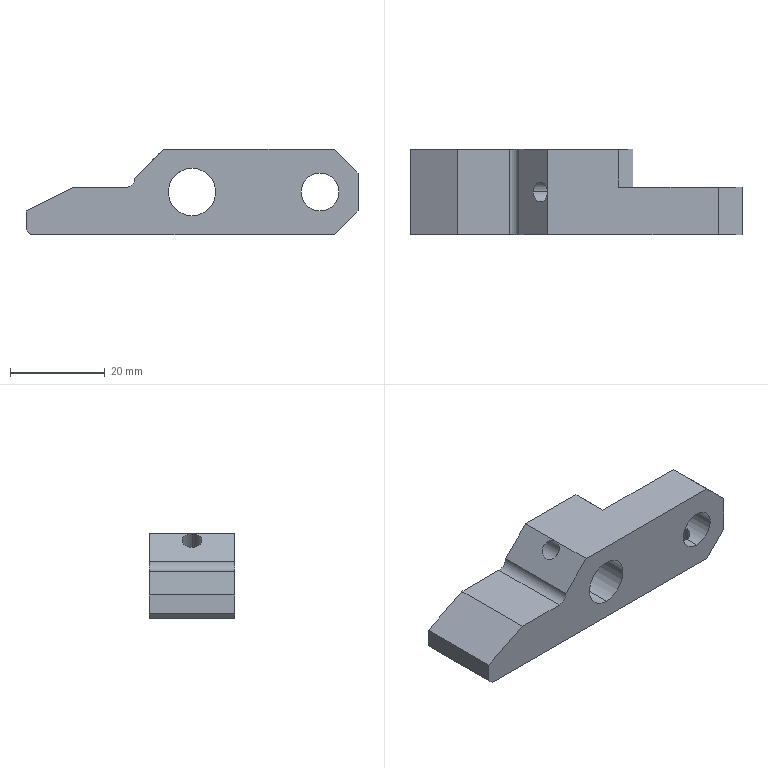Part | SolidWorks | features Chamfer 5, ICE 4, HoleWzd 3, 3DProfileFeature 1, CirPattern 1, Extrusion 1, Fillet 1 | 1 solid | 27 faces | box 70 x 18 x 18 mm | volume 12843 mm3 | plane 16 | cylinder 11 | commonest cylinder face diameters 4.2 x6 8 x2 10 x2 4 x1
STEP:
#1=CARTESIAN_POINT('',(-12.194,9.,1.724));
#2=VERTEX_POINT('',#1);
#3=CARTESIAN_POINT('',(-9.224,9.,4.694));
#4=VERTEX_POINT('',#3);
#5=CARTESIAN_POINT('',(-12.194,9.,1.724));
#6=CARTESIAN_POINT('',(-12.194,8.862,1.724));
#7=CARTESIAN_POINT('',(-12.188,8.721,1.738));
#8=CARTESIAN_POINT('',(-12.167,8.449,1.794));
#9=CARTESIAN_POINT('',(-12.151,8.318,1.836));
#10=CARTESIAN_POINT('',(-12.086,7.937,1.995));
#11=CARTESIAN_POINT('',(-12.02,7.708,2.147));
#12=CARTESIAN_POINT('',(-11.879,7.418,2.416));
#13=CARTESIAN_POINT('',(-11.826,7.332,2.511));
#14=CARTESIAN_POINT('',(-11.705,7.181,2.708));
#15=CARTESIAN_POINT('',(-11.636,7.115,2.813));
#16=CARTESIAN_POINT('',(-11.486,7.009,3.021));
#17=CARTESIAN_POINT('',(-11.405,6.969,3.126));
#18=CARTESIAN_POINT('',(-11.229,6.914,3.334));
#19=CARTESIAN_POINT('',(-11.134,6.9,3.437));
#20=CARTESIAN_POINT('',(-10.84,6.9,3.731));
#21=CARTESIAN_POINT('',(-10.625,6.956,3.911));
#22=CARTESIAN_POINT('',(-10.313,7.115,4.136));
#23=CARTESIAN_POINT('',(-10.208,7.181,4.205));
#24=CARTESIAN_POINT('',(-10.01,7.333,4.326));
#25=CARTESIAN_POINT('',(-9.915,7.419,4.379));
#26=CARTESIAN_POINT('',(-9.736,7.612,4.473));
#27=CARTESIAN_POINT('',(-9.653,7.718,4.513));
#28=CARTESIAN_POINT('',(-9.507,7.943,4.58));
#29=CARTESIAN_POINT('',(-9.443,8.063,4.608));
#30=CARTESIAN_POINT('',(-9.335,8.319,4.651));
#31=CARTESIAN_POINT('',(-9.294,8.45,4.667));
#32=CARTESIAN_POINT('',(-9.238,8.72,4.688));
#33=CARTESIAN_POINT('',(-9.224,8.86,4.694));
#34=CARTESIAN_POINT('',(-9.224,9.,4.694));
#35=B_SPLINE_CURVE_WITH_KNOTS('',3,(#5,#6,#7,#8,#9,#10,#11,#12,#13,#14,#15,#16,#17,#18,#19,#20,#21,#22,#23,#24,#25,#26,#27,#28,#29,#30,#31,#32,#33,#34),.UNSPECIFIED.,.F.,.F.,(4,2,2,2,2,2,2,2,2,2,2,2,2,2,4),(0.006643,0.007058,0.007473,0.008303,0.008717,0.009132,0.009547,0.009962,0.01079,0.01121,0.01162,0.01204,0.01245,0.01287,0.01328),.UNSPECIFIED.);
#36=EDGE_CURVE('',#2,#4,#35,.T.);
#37=ORIENTED_EDGE('',*,*,#36,.F.);
#38=CARTESIAN_POINT('',(-16.485,9.,6.015));
#39=VERTEX_POINT('',#38);
#40=CARTESIAN_POINT('',(-15.349,9.,4.879));
#41=DIRECTION('',(-0.7071,0.,0.7071));
#42=VECTOR('',#41,1000.);
#43=LINE('',#40,#42);
#44=EDGE_CURVE('',#2,#39,#43,.T.);
#45=ORIENTED_EDGE('',*,*,#44,.T.);
#46=CARTESIAN_POINT('',(-13.515,9.,8.985));
#47=VERTEX_POINT('',#46);
#48=CARTESIAN_POINT('',(-15.,9.,7.5));
#49=DIRECTION('',(-0.7071,0.,0.7071));
#50=DIRECTION('',(0.7071,0.,0.7071));
#51=AXIS2_PLACEMENT_3D('',#48,#49,#50);
#52=CIRCLE('',#51,2.1);
#53=EDGE_CURVE('',#39,#47,#52,.T.);
#54=ORIENTED_EDGE('',*,*,#53,.T.);
#55=CARTESIAN_POINT('',(-12.379,9.,7.849));
#56=DIRECTION('',(-0.7071,0.,0.7071));
#57=VECTOR('',#56,1000.);
#58=LINE('',#55,#57);
#59=EDGE_CURVE('',#4,#47,#58,.T.);
#60=ORIENTED_EDGE('',*,*,#59,.F.);
#61=EDGE_LOOP('',(#37,#45,#54,#60));
#62=FACE_OUTER_BOUND('',#61,.T.);
#63=CARTESIAN_POINT('',(-13.864,9.,6.364));
#64=DIRECTION('',(-0.7071,0.,0.7071));
#65=DIRECTION('',(0.7071,0.,0.7071));
#66=AXIS2_PLACEMENT_3D('',#63,#64,#65);
#67=CYLINDRICAL_SURFACE('',#66,2.1);
#68=ADVANCED_FACE('',(#62),#67,.F.);
#69=CARTESIAN_POINT('',(-5.4,9.,-4.538));
#70=VERTEX_POINT('',#69);
#71=CARTESIAN_POINT('',(-7.5,6.9,-5.));
#72=VERTEX_POINT('',#71);
#73=CARTESIAN_POINT('',(-5.4,9.,-4.538));
#74=CARTESIAN_POINT('',(-5.4,8.862,-4.538));
#75=CARTESIAN_POINT('',(-5.414,8.721,-4.544));
#76=CARTESIAN_POINT('',(-5.469,8.449,-4.569));
#77=CARTESIAN_POINT('',(-5.509,8.318,-4.587));
#78=CARTESIAN_POINT('',(-5.668,7.937,-4.654));
#79=CARTESIAN_POINT('',(-5.822,7.708,-4.715));
#80=CARTESIAN_POINT('',(-6.112,7.418,-4.805));
#81=CARTESIAN_POINT('',(-6.217,7.332,-4.834));
#82=CARTESIAN_POINT('',(-6.442,7.181,-4.888));
#83=CARTESIAN_POINT('',(-6.565,7.115,-4.913));
#84=CARTESIAN_POINT('',(-6.818,7.009,-4.955));
#85=CARTESIAN_POINT('',(-6.949,6.969,-4.971));
#86=CARTESIAN_POINT('',(-7.221,6.914,-4.994));
#87=CARTESIAN_POINT('',(-7.362,6.9,-5.));
#88=CARTESIAN_POINT('',(-7.5,6.9,-5.));
#89=B_SPLINE_CURVE_WITH_KNOTS('',3,(#73,#74,#75,#76,#77,#78,#79,#80,#81,#82,#83,#84,#85,#86,#87,#88),.UNSPECIFIED.,.F.,.F.,(4,2,2,2,2,2,2,4),(0.006643,0.007058,0.007473,0.008303,0.008718,0.009133,0.009547,0.009962),.UNSPECIFIED.);
#90=EDGE_CURVE('',#70,#72,#89,.T.);
#91=ORIENTED_EDGE('',*,*,#90,.F.);
#92=CARTESIAN_POINT('',(-5.4,9.,-9.));
#93=VERTEX_POINT('',#92);
#94=CARTESIAN_POINT('',(-5.4,9.,-9.));
#95=DIRECTION('',(0.,0.,-1.));
#96=VECTOR('',#95,1000.);
#97=LINE('',#94,#96);
#98=EDGE_CURVE('',#70,#93,#97,.T.);
#99=ORIENTED_EDGE('',*,*,#98,.T.);
#100=CARTESIAN_POINT('',(-9.6,9.,-9.));
#101=VERTEX_POINT('',#100);
#102=CARTESIAN_POINT('',(-7.5,9.,-9.));
#103=DIRECTION('',(0.,0.,-1.));
#104=DIRECTION('',(-1.,0.,0.));
#105=AXIS2_PLACEMENT_3D('',#102,#103,#104);
#106=CIRCLE('',#105,2.1);
#107=EDGE_CURVE('',#93,#101,#106,.T.);
#108=ORIENTED_EDGE('',*,*,#107,.T.);
#109=CARTESIAN_POINT('',(-9.6,9.,-4.538));
#110=VERTEX_POINT('',#109);
#111=CARTESIAN_POINT('',(-9.6,9.,-9.));
#112=DIRECTION('',(0.,0.,-1.));
#113=VECTOR('',#112,1000.);
#114=LINE('',#111,#113);
#115=EDGE_CURVE('',#110,#101,#114,.T.);
#116=ORIENTED_EDGE('',*,*,#115,.F.);
#117=CARTESIAN_POINT('',(-7.5,6.9,-5.));
#118=CARTESIAN_POINT('',(-7.777,6.9,-5.));
#119=CARTESIAN_POINT('',(-8.056,6.956,-4.976));
#120=CARTESIAN_POINT('',(-8.436,7.115,-4.913));
#121=CARTESIAN_POINT('',(-8.558,7.181,-4.888));
#122=CARTESIAN_POINT('',(-8.784,7.333,-4.834));
#123=CARTESIAN_POINT('',(-8.889,7.419,-4.804));
#124=CARTESIAN_POINT('',(-9.082,7.612,-4.744));
#125=CARTESIAN_POINT('',(-9.169,7.718,-4.714));
#126=CARTESIAN_POINT('',(-9.32,7.943,-4.658));
#127=CARTESIAN_POINT('',(-9.385,8.063,-4.632));
#128=CARTESIAN_POINT('',(-9.491,8.319,-4.587));
#129=CARTESIAN_POINT('',(-9.531,8.45,-4.569));
#130=CARTESIAN_POINT('',(-9.586,8.72,-4.544));
#131=CARTESIAN_POINT('',(-9.6,8.86,-4.538));
#132=CARTESIAN_POINT('',(-9.6,9.,-4.538));
#133=B_SPLINE_CURVE_WITH_KNOTS('',3,(#117,#118,#119,#120,#121,#122,#123,#124,#125,#126,#127,#128,#129,#130,#131,#132),.UNSPECIFIED.,.F.,.F.,(4,2,2,2,2,2,2,4),(0.009962,0.01079,0.01121,0.01162,0.01204,0.01245,0.01287,0.01328),.UNSPECIFIED.);
#134=EDGE_CURVE('',#72,#110,#133,.T.);
#135=ORIENTED_EDGE('',*,*,#134,.F.);
#136=EDGE_LOOP('',(#91,#99,#108,#116,#135));
#137=FACE_OUTER_BOUND('',#136,.T.);
#138=CARTESIAN_POINT('',(-7.5,9.,-9.));
#139=DIRECTION('',(0.,0.,-1.));
#140=DIRECTION('',(-1.,0.,0.));
#141=AXIS2_PLACEMENT_3D('',#138,#139,#140);
#142=CYLINDRICAL_SURFACE('',#141,2.1);
#143=ADVANCED_FACE('',(#137),#142,.F.);
#144=CARTESIAN_POINT('',(19.5,2.9,-4.));
#145=VERTEX_POINT('',#144);
#146=CARTESIAN_POINT('',(21.6,5.,-3.404));
#147=VERTEX_POINT('',#146);
#148=CARTESIAN_POINT('',(19.5,2.9,-4.));
#149=CARTESIAN_POINT('',(19.64,2.9,-4.));
#150=CARTESIAN_POINT('',(19.782,2.914,-3.992));
#151=CARTESIAN_POINT('',(20.054,2.97,-3.964));
#152=CARTESIAN_POINT('',(20.187,3.011,-3.943));
#153=CARTESIAN_POINT('',(20.443,3.118,-3.89));
#154=CARTESIAN_POINT('',(20.563,3.184,-3.858));
#155=CARTESIAN_POINT('',(20.788,3.335,-3.789));
#156=CARTESIAN_POINT('',(20.893,3.423,-3.751));
#157=CARTESIAN_POINT('',(21.083,3.614,-3.675));
#158=CARTESIAN_POINT('',(21.168,3.718,-3.636));
#159=CARTESIAN_POINT('',(21.32,3.943,-3.563));
#160=CARTESIAN_POINT('',(21.385,4.064,-3.529));
#161=CARTESIAN_POINT('',(21.542,4.44,-3.441));
#162=CARTESIAN_POINT('',(21.6,4.721,-3.404));
#163=CARTESIAN_POINT('',(21.6,5.,-3.404));
#164=B_SPLINE_CURVE_WITH_KNOTS('',3,(#148,#149,#150,#151,#152,#153,#154,#155,#156,#157,#158,#159,#160,#161,#162,#163),.UNSPECIFIED.,.F.,.F.,(4,2,2,2,2,2,2,4),(0.006693,0.007111,0.007529,0.007947,0.008365,0.008783,0.0092,0.01004),.UNSPECIFIED.);
#165=EDGE_CURVE('',#145,#147,#164,.T.);
#166=ORIENTED_EDGE('',*,*,#165,.T.);
#167=CARTESIAN_POINT('',(21.6,5.,-9.));
#168=VERTEX_POINT('',#167);
#169=CARTESIAN_POINT('',(21.6,5.,-9.));
#170=DIRECTION('',(0.,0.,-1.));
#171=VECTOR('',#170,1000.);
#172=LINE('',#169,#171);
#173=EDGE_CURVE('',#147,#168,#172,.T.);
#174=ORIENTED_EDGE('',*,*,#173,.T.);
#175=CARTESIAN_POINT('',(17.4,5.,-9.));
#176=VERTEX_POINT('',#175);
#177=CARTESIAN_POINT('',(19.5,5.,-9.));
#178=DIRECTION('',(0.,0.,-1.));
#179=DIRECTION('',(-1.,0.,0.));
#180=AXIS2_PLACEMENT_3D('',#177,#178,#179);
#181=CIRCLE('',#180,2.1);
#182=EDGE_CURVE('',#168,#176,#181,.T.);
#183=ORIENTED_EDGE('',*,*,#182,.T.);
#184=CARTESIAN_POINT('',(17.4,5.,-3.404));
#185=VERTEX_POINT('',#184);
#186=CARTESIAN_POINT('',(17.4,5.,-9.));
#187=DIRECTION('',(0.,0.,-1.));
#188=VECTOR('',#187,1000.);
#189=LINE('',#186,#188);
#190=EDGE_CURVE('',#185,#176,#189,.T.);
#191=ORIENTED_EDGE('',*,*,#190,.F.);
#192=CARTESIAN_POINT('',(17.4,5.,-3.404));
#193=CARTESIAN_POINT('',(17.4,4.86,-3.404));
#194=CARTESIAN_POINT('',(17.414,4.718,-3.413));
#195=CARTESIAN_POINT('',(17.47,4.446,-3.446));
#196=CARTESIAN_POINT('',(17.511,4.313,-3.471));
#197=CARTESIAN_POINT('',(17.617,4.059,-3.53));
#198=CARTESIAN_POINT('',(17.682,3.94,-3.564));
#199=CARTESIAN_POINT('',(17.834,3.715,-3.637));
#200=CARTESIAN_POINT('',(17.92,3.61,-3.676));
#201=CARTESIAN_POINT('',(18.205,3.325,-3.79));
#202=CARTESIAN_POINT('',(18.436,3.169,-3.864));
#203=CARTESIAN_POINT('',(18.814,3.011,-3.943));
#204=CARTESIAN_POINT('',(18.948,2.969,-3.964));
#205=CARTESIAN_POINT('',(19.222,2.914,-3.993));
#206=CARTESIAN_POINT('',(19.36,2.9,-4.));
#207=CARTESIAN_POINT('',(19.5,2.9,-4.));
#208=B_SPLINE_CURVE_WITH_KNOTS('',3,(#192,#193,#194,#195,#196,#197,#198,#199,#200,#201,#202,#203,#204,#205,#206,#207),.UNSPECIFIED.,.F.,.F.,(4,2,2,2,2,2,2,4),(0.003349,0.003767,0.004185,0.004603,0.005021,0.005857,0.006275,0.006693),.UNSPECIFIED.);
#209=EDGE_CURVE('',#185,#145,#208,.T.);
#210=ORIENTED_EDGE('',*,*,#209,.T.);
#211=EDGE_LOOP('',(#166,#174,#183,#191,#210));
#212=FACE_OUTER_BOUND('',#211,.T.);
#213=CARTESIAN_POINT('',(19.5,5.,-9.));
#214=DIRECTION('',(0.,0.,-1.));
#215=DIRECTION('',(-1.,0.,0.));
#216=AXIS2_PLACEMENT_3D('',#213,#214,#215);
#217=CYLINDRICAL_SURFACE('',#216,2.1);
#218=ADVANCED_FACE('',(#212),#217,.F.);
#219=CARTESIAN_POINT('',(-9.224,9.,4.694));
#220=CARTESIAN_POINT('',(-9.224,9.141,4.694));
#221=CARTESIAN_POINT('',(-9.238,9.278,4.688));
#222=CARTESIAN_POINT('',(-9.294,9.549,4.667));
#223=CARTESIAN_POINT('',(-9.336,9.683,4.651));
#224=CARTESIAN_POINT('',(-9.442,9.936,4.608));
#225=CARTESIAN_POINT('',(-9.506,10.056,4.58));
#226=CARTESIAN_POINT('',(-9.654,10.283,4.513));
#227=CARTESIAN_POINT('',(-9.737,10.389,4.473));
#228=CARTESIAN_POINT('',(-10.003,10.676,4.333));
#229=CARTESIAN_POINT('',(-10.209,10.832,4.211));
#230=CARTESIAN_POINT('',(-10.52,10.99,3.987));
#231=CARTESIAN_POINT('',(-10.627,11.032,3.904));
#232=CARTESIAN_POINT('',(-10.835,11.086,3.728));
#233=CARTESIAN_POINT('',(-10.936,11.1,3.635));
#234=CARTESIAN_POINT('',(-11.133,11.1,3.438));
#235=CARTESIAN_POINT('',(-11.228,11.086,3.334));
#236=CARTESIAN_POINT('',(-11.404,11.032,3.127));
#237=CARTESIAN_POINT('',(-11.486,10.991,3.022));
#238=CARTESIAN_POINT('',(-11.637,10.884,2.811));
#239=CARTESIAN_POINT('',(-11.705,10.819,2.708));
#240=CARTESIAN_POINT('',(-11.826,10.667,2.51));
#241=CARTESIAN_POINT('',(-11.88,10.579,2.413));
#242=CARTESIAN_POINT('',(-11.973,10.387,2.236));
#243=CARTESIAN_POINT('',(-12.013,10.283,2.154));
#244=CARTESIAN_POINT('',(-12.081,10.056,2.006));
#245=CARTESIAN_POINT('',(-12.108,9.934,1.941));
#246=CARTESIAN_POINT('',(-12.173,9.556,1.783));
#247=CARTESIAN_POINT('',(-12.194,9.277,1.724));
#248=CARTESIAN_POINT('',(-12.194,9.,1.724));
#249=B_SPLINE_CURVE_WITH_KNOTS('',3,(#219,#220,#221,#222,#223,#224,#225,#226,#227,#228,#229,#230,#231,#232,#233,#234,#235,#236,#237,#238,#239,#240,#241,#242,#243,#244,#245,#246,#247,#248),.UNSPECIFIED.,.F.,.F.,(4,2,2,2,2,2,2,2,2,2,2,2,2,2,4),(0.,0.0004152,0.0008304,0.001246,0.001661,0.002491,0.002906,0.003322,0.003737,0.004152,0.004567,0.004982,0.005398,0.005813,0.006643),.UNSPECIFIED.);
#250=EDGE_CURVE('',#4,#2,#249,.T.);
#251=ORIENTED_EDGE('',*,*,#250,.T.);
#252=ORIENTED_EDGE('',*,*,#36,.T.);
#253=EDGE_LOOP('',(#251,#252));
#254=FACE_BOUND('',#253,.T.);
#255=CARTESIAN_POINT('',(-7.5,0.,5.));
#256=VERTEX_POINT('',#255);
#257=CARTESIAN_POINT('',(-7.5,0.,-5.));
#258=VERTEX_POINT('',#257);
#259=CARTESIAN_POINT('',(-7.5,0.,0.));
#260=DIRECTION('',(0.,-1.,0.));
#261=DIRECTION('',(0.,0.,-1.));
#262=AXIS2_PLACEMENT_3D('',#259,#260,#261);
#263=CIRCLE('',#262,5.);
#264=EDGE_CURVE('',#256,#258,#263,.T.);
#265=ORIENTED_EDGE('',*,*,#264,.T.);
#266=CARTESIAN_POINT('',(-7.5,-9.,-5.));
#267=DIRECTION('',(0.,1.,0.));
#268=VECTOR('',#267,1000.);
#269=LINE('',#266,#268);
#270=EDGE_CURVE('',#258,#72,#269,.T.);
#271=ORIENTED_EDGE('',*,*,#270,.T.);
#272=ORIENTED_EDGE('',*,*,#134,.T.);
#273=CARTESIAN_POINT('',(-7.5,11.1,-5.));
#274=VERTEX_POINT('',#273);
#275=CARTESIAN_POINT('',(-9.6,9.,-4.538));
#276=CARTESIAN_POINT('',(-9.6,9.141,-4.538));
#277=CARTESIAN_POINT('',(-9.586,9.278,-4.544));
#278=CARTESIAN_POINT('',(-9.532,9.549,-4.569));
#279=CARTESIAN_POINT('',(-9.49,9.683,-4.587));
#280=CARTESIAN_POINT('',(-9.385,9.937,-4.632));
#281=CARTESIAN_POINT('',(-9.32,10.057,-4.658));
#282=CARTESIAN_POINT('',(-9.168,10.284,-4.714));
#283=CARTESIAN_POINT('',(-9.08,10.39,-4.745));
#284=CARTESIAN_POINT('',(-8.793,10.677,-4.834));
#285=CARTESIAN_POINT('',(-8.561,10.833,-4.893));
#286=CARTESIAN_POINT('',(-8.183,10.991,-4.955));
#287=CARTESIAN_POINT('',(-8.049,11.032,-4.972));
#288=CARTESIAN_POINT('',(-7.776,11.086,-4.994));
#289=CARTESIAN_POINT('',(-7.639,11.1,-5.));
#290=CARTESIAN_POINT('',(-7.5,11.1,-5.));
#291=B_SPLINE_CURVE_WITH_KNOTS('',3,(#275,#276,#277,#278,#279,#280,#281,#282,#283,#284,#285,#286,#287,#288,#289,#290),.UNSPECIFIED.,.F.,.F.,(4,2,2,2,2,2,2,4),(0.,0.0004153,0.0008307,0.001246,0.001661,0.002492,0.002907,0.003323),.UNSPECIFIED.);
#292=EDGE_CURVE('',#110,#274,#291,.T.);
#293=ORIENTED_EDGE('',*,*,#292,.T.);
#294=CARTESIAN_POINT('',(-7.5,18.,-5.));
#295=VERTEX_POINT('',#294);
#296=CARTESIAN_POINT('',(-7.5,-9.,-5.));
#297=DIRECTION('',(0.,1.,0.));
#298=VECTOR('',#297,1000.);
#299=LINE('',#296,#298);
#300=EDGE_CURVE('',#274,#295,#299,.T.);
#301=ORIENTED_EDGE('',*,*,#300,.T.);
#302=CARTESIAN_POINT('',(-7.5,18.,5.));
#303=VERTEX_POINT('',#302);
#304=CARTESIAN_POINT('',(-7.5,18.,0.));
#305=DIRECTION('',(0.,1.,0.));
#306=DIRECTION('',(0.,0.,1.));
#307=AXIS2_PLACEMENT_3D('',#304,#305,#306);
#308=CIRCLE('',#307,5.);
#309=EDGE_CURVE('',#295,#303,#308,.T.);
#310=ORIENTED_EDGE('',*,*,#309,.T.);
#311=CARTESIAN_POINT('',(-7.5,-9.,5.));
#312=DIRECTION('',(0.,1.,0.));
#313=VECTOR('',#312,1000.);
#314=LINE('',#311,#313);
#315=EDGE_CURVE('',#256,#303,#314,.T.);
#316=ORIENTED_EDGE('',*,*,#315,.F.);
#317=EDGE_LOOP('',(#265,#271,#272,#293,#301,#310,#316));
#318=FACE_OUTER_BOUND('',#317,.T.);
#319=CARTESIAN_POINT('',(-7.5,-9.,0.));
#320=DIRECTION('',(0.,1.,0.));
#321=DIRECTION('',(0.,0.,1.));
#322=AXIS2_PLACEMENT_3D('',#319,#320,#321);
#323=CYLINDRICAL_SURFACE('',#322,5.);
#324=ADVANCED_FACE('',(#254,#318),#323,.F.);
#325=CARTESIAN_POINT('',(19.5,10.,-4.));
#326=VERTEX_POINT('',#325);
#327=CARTESIAN_POINT('',(19.5,10.,4.));
#328=VERTEX_POINT('',#327);
#329=CARTESIAN_POINT('',(19.5,10.,0.));
#330=DIRECTION('',(0.,1.,0.));
#331=DIRECTION('',(0.,0.,1.));
#332=AXIS2_PLACEMENT_3D('',#329,#330,#331);
#333=CIRCLE('',#332,4.);
#334=EDGE_CURVE('',#326,#328,#333,.T.);
#335=ORIENTED_EDGE('',*,*,#334,.T.);
#336=CARTESIAN_POINT('',(19.5,0.,4.));
#337=VERTEX_POINT('',#336);
#338=CARTESIAN_POINT('',(19.5,10.,4.));
#339=DIRECTION('',(0.,-1.,0.));
#340=VECTOR('',#339,1000.);
#341=LINE('',#338,#340);
#342=EDGE_CURVE('',#328,#337,#341,.T.);
#343=ORIENTED_EDGE('',*,*,#342,.T.);
#344=CARTESIAN_POINT('',(19.5,0.,-4.));
#345=VERTEX_POINT('',#344);
#346=CARTESIAN_POINT('',(19.5,0.,0.));
#347=DIRECTION('',(0.,1.,0.));
#348=DIRECTION('',(0.,0.,1.));
#349=AXIS2_PLACEMENT_3D('',#346,#347,#348);
#350=CIRCLE('',#349,4.);
#351=EDGE_CURVE('',#345,#337,#350,.T.);
#352=ORIENTED_EDGE('',*,*,#351,.F.);
#353=CARTESIAN_POINT('',(19.5,10.,-4.));
#354=DIRECTION('',(0.,-1.,0.));
#355=VECTOR('',#354,1000.);
#356=LINE('',#353,#355);
#357=EDGE_CURVE('',#145,#345,#356,.T.);
#358=ORIENTED_EDGE('',*,*,#357,.F.);
#359=ORIENTED_EDGE('',*,*,#209,.F.);
#360=CARTESIAN_POINT('',(19.5,7.1,-4.));
#361=VERTEX_POINT('',#360);
#362=CARTESIAN_POINT('',(19.5,7.1,-4.));
#363=CARTESIAN_POINT('',(19.358,7.1,-4.));
#364=CARTESIAN_POINT('',(19.219,7.086,-3.992));
#365=CARTESIAN_POINT('',(18.947,7.031,-3.964));
#366=CARTESIAN_POINT('',(18.812,6.989,-3.943));
#367=CARTESIAN_POINT('',(18.432,6.829,-3.863));
#368=CARTESIAN_POINT('',(18.202,6.673,-3.789));
#369=CARTESIAN_POINT('',(17.917,6.387,-3.675));
#370=CARTESIAN_POINT('',(17.831,6.282,-3.636));
#371=CARTESIAN_POINT('',(17.68,6.056,-3.563));
#372=CARTESIAN_POINT('',(17.616,5.937,-3.529));
#373=CARTESIAN_POINT('',(17.51,5.685,-3.471));
#374=CARTESIAN_POINT('',(17.469,5.551,-3.446));
#375=CARTESIAN_POINT('',(17.414,5.278,-3.413));
#376=CARTESIAN_POINT('',(17.4,5.14,-3.404));
#377=CARTESIAN_POINT('',(17.4,5.,-3.404));
#378=B_SPLINE_CURVE_WITH_KNOTS('',3,(#362,#363,#364,#365,#366,#367,#368,#369,#370,#371,#372,#373,#374,#375,#376,#377),.UNSPECIFIED.,.F.,.F.,(4,2,2,2,2,2,2,4),(0.,0.0004186,0.0008373,0.001675,0.002093,0.002512,0.00293,0.003349),.UNSPECIFIED.);
#379=EDGE_CURVE('',#361,#185,#378,.T.);
#380=ORIENTED_EDGE('',*,*,#379,.F.);
#381=CARTESIAN_POINT('',(19.5,10.,-4.));
#382=DIRECTION('',(0.,-1.,0.));
#383=VECTOR('',#382,1000.);
#384=LINE('',#381,#383);
#385=EDGE_CURVE('',#326,#361,#384,.T.);
#386=ORIENTED_EDGE('',*,*,#385,.F.);
#387=EDGE_LOOP('',(#335,#343,#352,#358,#359,#380,#386));
#388=FACE_OUTER_BOUND('',#387,.T.);
#389=CARTESIAN_POINT('',(19.5,10.,0.));
#390=DIRECTION('',(0.,-1.,0.));
#391=DIRECTION('',(0.,0.,-1.));
#392=AXIS2_PLACEMENT_3D('',#389,#390,#391);
#393=CYLINDRICAL_SURFACE('',#392,4.);
#394=ADVANCED_FACE('',(#388),#393,.F.);
#395=ORIENTED_EDGE('',*,*,#334,.F.);
#396=CARTESIAN_POINT('',(19.5,10.,0.));
#397=DIRECTION('',(0.,1.,0.));
#398=DIRECTION('',(0.,0.,1.));
#399=AXIS2_PLACEMENT_3D('',#396,#397,#398);
#400=CIRCLE('',#399,4.);
#401=EDGE_CURVE('',#328,#326,#400,.T.);
#402=ORIENTED_EDGE('',*,*,#401,.F.);
#403=EDGE_LOOP('',(#395,#402));
#404=FACE_BOUND('',#403,.T.);
#405=CARTESIAN_POINT('',(27.5,10.,4.));
#406=VERTEX_POINT('',#405);
#407=CARTESIAN_POINT('',(27.5,10.,-4.));
#408=VERTEX_POINT('',#407);
#409=CARTESIAN_POINT('',(27.5,10.,-9.));
#410=DIRECTION('',(0.,0.,-1.));
#411=VECTOR('',#410,1000.);
#412=LINE('',#409,#411);
#413=EDGE_CURVE('',#406,#408,#412,.T.);
#414=ORIENTED_EDGE('',*,*,#413,.T.);
#415=CARTESIAN_POINT('',(22.5,10.,-9.));
#416=VERTEX_POINT('',#415);
#417=CARTESIAN_POINT('',(22.5,10.,-9.));
#418=DIRECTION('',(-0.7071,0.,-0.7071));
#419=VECTOR('',#418,1000.);
#420=LINE('',#417,#419);
#421=EDGE_CURVE('',#408,#416,#420,.T.);
#422=ORIENTED_EDGE('',*,*,#421,.T.);
#423=CARTESIAN_POINT('',(1.5,10.,-9.));
#424=VERTEX_POINT('',#423);
#425=CARTESIAN_POINT('',(27.5,10.,-9.));
#426=DIRECTION('',(-1.,0.,0.));
#427=VECTOR('',#426,1000.);
#428=LINE('',#425,#427);
#429=EDGE_CURVE('',#416,#424,#428,.T.);
#430=ORIENTED_EDGE('',*,*,#429,.T.);
#431=CARTESIAN_POINT('',(4.5,10.,-6.));
#432=VERTEX_POINT('',#431);
#433=CARTESIAN_POINT('',(5.25,10.,-5.25));
#434=DIRECTION('',(0.7071,0.,0.7071));
#435=VECTOR('',#434,1000.);
#436=LINE('',#433,#435);
#437=EDGE_CURVE('',#424,#432,#436,.T.);
#438=ORIENTED_EDGE('',*,*,#437,.T.);
#439=CARTESIAN_POINT('',(4.5,10.,6.));
#440=VERTEX_POINT('',#439);
#441=CARTESIAN_POINT('',(4.5,10.,41.985));
#442=DIRECTION('',(0.,0.,-1.));
#443=VECTOR('',#442,1000.);
#444=LINE('',#441,#443);
#445=EDGE_CURVE('',#440,#432,#444,.T.);
#446=ORIENTED_EDGE('',*,*,#445,.F.);
#447=CARTESIAN_POINT('',(1.5,10.,9.));
#448=VERTEX_POINT('',#447);
#449=CARTESIAN_POINT('',(5.25,10.,5.25));
#450=DIRECTION('',(-0.7071,0.,0.7071));
#451=VECTOR('',#450,1000.);
#452=LINE('',#449,#451);
#453=EDGE_CURVE('',#440,#448,#452,.T.);
#454=ORIENTED_EDGE('',*,*,#453,.T.);
#455=CARTESIAN_POINT('',(22.5,10.,9.));
#456=VERTEX_POINT('',#455);
#457=CARTESIAN_POINT('',(27.5,10.,9.));
#458=DIRECTION('',(1.,0.,0.));
#459=VECTOR('',#458,1000.);
#460=LINE('',#457,#459);
#461=EDGE_CURVE('',#448,#456,#460,.T.);
#462=ORIENTED_EDGE('',*,*,#461,.T.);
#463=CARTESIAN_POINT('',(27.5,10.,4.));
#464=DIRECTION('',(0.7071,0.,-0.7071));
#465=VECTOR('',#464,1000.);
#466=LINE('',#463,#465);
#467=EDGE_CURVE('',#456,#406,#466,.T.);
#468=ORIENTED_EDGE('',*,*,#467,.T.);
#469=EDGE_LOOP('',(#414,#422,#430,#438,#446,#454,#462,#468));
#470=FACE_OUTER_BOUND('',#469,.T.);
#471=CARTESIAN_POINT('',(0.,10.,0.));
#472=DIRECTION('',(0.,-1.,0.));
#473=DIRECTION('',(0.,0.,-1.));
#474=AXIS2_PLACEMENT_3D('',#471,#472,#473);
#475=PLANE('',#474);
#476=ADVANCED_FACE('',(#404,#470),#475,.F.);
#477=CARTESIAN_POINT('',(-42.5,0.,-8.));
#478=VERTEX_POINT('',#477);
#479=CARTESIAN_POINT('',(-42.5,0.,-4.));
#480=VERTEX_POINT('',#479);
#481=CARTESIAN_POINT('',(-42.5,0.,-9.));
#482=DIRECTION('',(0.,0.,1.));
#483=VECTOR('',#482,1000.);
#484=LINE('',#481,#483);
#485=EDGE_CURVE('',#478,#480,#484,.T.);
#486=ORIENTED_EDGE('',*,*,#485,.F.);
#487=CARTESIAN_POINT('',(-41.5,0.,-9.));
#488=VERTEX_POINT('',#487);
#489=CARTESIAN_POINT('',(-25.25,0.,-25.25));
#490=DIRECTION('',(0.7071,0.,-0.7071));
#491=VECTOR('',#490,1000.);
#492=LINE('',#489,#491);
#493=EDGE_CURVE('',#478,#488,#492,.T.);
#494=ORIENTED_EDGE('',*,*,#493,.T.);
#495=CARTESIAN_POINT('',(22.5,0.,-9.));
#496=VERTEX_POINT('',#495);
#497=CARTESIAN_POINT('',(27.5,0.,-9.));
#498=DIRECTION('',(-1.,0.,0.));
#499=VECTOR('',#498,1000.);
#500=LINE('',#497,#499);
#501=EDGE_CURVE('',#496,#488,#500,.T.);
#502=ORIENTED_EDGE('',*,*,#501,.F.);
#503=CARTESIAN_POINT('',(27.5,0.,-4.));
#504=VERTEX_POINT('',#503);
#505=CARTESIAN_POINT('',(15.75,0.,-15.75));
#506=DIRECTION('',(0.7071,0.,0.7071));
#507=VECTOR('',#506,1000.);
#508=LINE('',#505,#507);
#509=EDGE_CURVE('',#496,#504,#508,.T.);
#510=ORIENTED_EDGE('',*,*,#509,.T.);
#511=CARTESIAN_POINT('',(27.5,0.,4.));
#512=VERTEX_POINT('',#511);
#513=CARTESIAN_POINT('',(27.5,0.,-9.));
#514=DIRECTION('',(0.,0.,-1.));
#515=VECTOR('',#514,1000.);
#516=LINE('',#513,#515);
#517=EDGE_CURVE('',#512,#504,#516,.T.);
#518=ORIENTED_EDGE('',*,*,#517,.F.);
#519=CARTESIAN_POINT('',(22.5,0.,9.));
#520=VERTEX_POINT('',#519);
#521=CARTESIAN_POINT('',(15.75,0.,15.75));
#522=DIRECTION('',(-0.7071,0.,0.7071));
#523=VECTOR('',#522,1000.);
#524=LINE('',#521,#523);
#525=EDGE_CURVE('',#512,#520,#524,.T.);
#526=ORIENTED_EDGE('',*,*,#525,.T.);
#527=CARTESIAN_POINT('',(-13.5,0.,9.));
#528=VERTEX_POINT('',#527);
#529=CARTESIAN_POINT('',(27.5,0.,9.));
#530=DIRECTION('',(1.,0.,0.));
#531=VECTOR('',#530,1000.);
#532=LINE('',#529,#531);
#533=EDGE_CURVE('',#528,#520,#532,.T.);
#534=ORIENTED_EDGE('',*,*,#533,.F.);
#535=CARTESIAN_POINT('',(-19.5,0.,3.));
#536=VERTEX_POINT('',#535);
#537=CARTESIAN_POINT('',(-11.25,0.,11.25));
#538=DIRECTION('',(-0.7071,0.,-0.7071));
#539=VECTOR('',#538,1000.);
#540=LINE('',#537,#539);
#541=EDGE_CURVE('',#528,#536,#540,.T.);
#542=ORIENTED_EDGE('',*,*,#541,.T.);
#543=CARTESIAN_POINT('',(-21.5,0.,1.));
#544=VERTEX_POINT('',#543);
#545=CARTESIAN_POINT('',(-21.5,0.,3.));
#546=DIRECTION('',(0.,1.,0.));
#547=DIRECTION('',(0.,0.,-1.));
#548=AXIS2_PLACEMENT_3D('',#545,#546,#547);
#549=CIRCLE('',#548,2.);
#550=EDGE_CURVE('',#536,#544,#549,.T.);
#551=ORIENTED_EDGE('',*,*,#550,.T.);
#552=CARTESIAN_POINT('',(-32.5,0.,1.));
#553=VERTEX_POINT('',#552);
#554=CARTESIAN_POINT('',(-27.5,0.,1.));
#555=DIRECTION('',(1.,0.,0.));
#556=VECTOR('',#555,1000.);
#557=LINE('',#554,#556);
#558=EDGE_CURVE('',#553,#544,#557,.T.);
#559=ORIENTED_EDGE('',*,*,#558,.F.);
#560=CARTESIAN_POINT('',(-6.9,0.,13.8));
#561=DIRECTION('',(-0.8944,0.,-0.4472));
#562=VECTOR('',#561,1000.);
#563=LINE('',#560,#562);
#564=EDGE_CURVE('',#553,#480,#563,.T.);
#565=ORIENTED_EDGE('',*,*,#564,.T.);
#566=EDGE_LOOP('',(#486,#494,#502,#510,#518,#526,#534,#542,#551,#559,#565));
#567=FACE_OUTER_BOUND('',#566,.T.);
#568=ORIENTED_EDGE('',*,*,#264,.F.);
#569=CARTESIAN_POINT('',(-7.5,0.,0.));
#570=DIRECTION('',(0.,-1.,0.));
#571=DIRECTION('',(0.,0.,-1.));
#572=AXIS2_PLACEMENT_3D('',#569,#570,#571);
#573=CIRCLE('',#572,5.);
#574=EDGE_CURVE('',#258,#256,#573,.T.);
#575=ORIENTED_EDGE('',*,*,#574,.F.);
#576=EDGE_LOOP('',(#568,#575));
#577=FACE_BOUND('',#576,.T.);
#578=ORIENTED_EDGE('',*,*,#351,.T.);
#579=CARTESIAN_POINT('',(19.5,0.,0.));
#580=DIRECTION('',(0.,1.,0.));
#581=DIRECTION('',(0.,0.,1.));
#582=AXIS2_PLACEMENT_3D('',#579,#580,#581);
#583=CIRCLE('',#582,4.);
#584=EDGE_CURVE('',#337,#345,#583,.T.);
#585=ORIENTED_EDGE('',*,*,#584,.T.);
#586=EDGE_LOOP('',(#578,#585));
#587=FACE_BOUND('',#586,.T.);
#588=CARTESIAN_POINT('',(0.,0.,0.));
#589=DIRECTION('',(0.,-1.,0.));
#590=DIRECTION('',(0.,0.,-1.));
#591=AXIS2_PLACEMENT_3D('',#588,#589,#590);
#592=PLANE('',#591);
#593=ADVANCED_FACE('',(#567,#577,#587),#592,.T.);
#594=CARTESIAN_POINT('',(1.5,18.,9.));
#595=VERTEX_POINT('',#594);
#596=CARTESIAN_POINT('',(-13.5,18.,9.));
#597=VERTEX_POINT('',#596);
#598=CARTESIAN_POINT('',(-27.5,18.,9.));
#599=DIRECTION('',(-1.,0.,0.));
#600=VECTOR('',#599,1000.);
#601=LINE('',#598,#600);
#602=EDGE_CURVE('',#595,#597,#601,.T.);
#603=ORIENTED_EDGE('',*,*,#602,.T.);
#604=CARTESIAN_POINT('',(-13.5,10.,9.));
#605=DIRECTION('',(0.,-1.,0.));
#606=VECTOR('',#605,1000.);
#607=LINE('',#604,#606);
#608=EDGE_CURVE('',#597,#528,#607,.T.);
#609=ORIENTED_EDGE('',*,*,#608,.T.);
#610=ORIENTED_EDGE('',*,*,#533,.T.);
#611=CARTESIAN_POINT('',(22.5,10.,9.));
#612=DIRECTION('',(0.,1.,0.));
#613=VECTOR('',#612,1000.);
#614=LINE('',#611,#613);
#615=EDGE_CURVE('',#520,#456,#614,.T.);
#616=ORIENTED_EDGE('',*,*,#615,.T.);
#617=ORIENTED_EDGE('',*,*,#461,.F.);
#618=CARTESIAN_POINT('',(1.5,18.,9.));
#619=DIRECTION('',(0.,1.,0.));
#620=VECTOR('',#619,1000.);
#621=LINE('',#618,#620);
#622=EDGE_CURVE('',#448,#595,#621,.T.);
#623=ORIENTED_EDGE('',*,*,#622,.T.);
#624=EDGE_LOOP('',(#603,#609,#610,#616,#617,#623));
#625=FACE_OUTER_BOUND('',#624,.T.);
#626=CARTESIAN_POINT('',(27.5,10.,9.));
#627=DIRECTION('',(0.,0.,-1.));
#628=DIRECTION('',(-1.,0.,0.));
#629=AXIS2_PLACEMENT_3D('',#626,#627,#628);
#630=PLANE('',#629);
#631=ADVANCED_FACE('',(#625),#630,.F.);
#632=ORIENTED_EDGE('',*,*,#517,.T.);
#633=CARTESIAN_POINT('',(27.5,10.,-4.));
#634=DIRECTION('',(0.,1.,0.));
#635=VECTOR('',#634,1000.);
#636=LINE('',#633,#635);
#637=EDGE_CURVE('',#504,#408,#636,.T.);
#638=ORIENTED_EDGE('',*,*,#637,.T.);
#639=ORIENTED_EDGE('',*,*,#413,.F.);
#640=CARTESIAN_POINT('',(27.5,10.,4.));
#641=DIRECTION('',(0.,-1.,0.));
#642=VECTOR('',#641,1000.);
#643=LINE('',#640,#642);
#644=EDGE_CURVE('',#406,#512,#643,.T.);
#645=ORIENTED_EDGE('',*,*,#644,.T.);
#646=EDGE_LOOP('',(#632,#638,#639,#645));
#647=FACE_OUTER_BOUND('',#646,.T.);
#648=CARTESIAN_POINT('',(27.5,10.,-9.));
#649=DIRECTION('',(-1.,0.,0.));
#650=DIRECTION('',(0.,0.,1.));
#651=AXIS2_PLACEMENT_3D('',#648,#649,#650);
#652=PLANE('',#651);
#653=ADVANCED_FACE('',(#647),#652,.F.);
#654=CARTESIAN_POINT('',(-7.5,9.,-9.));
#655=DIRECTION('',(0.,0.,-1.));
#656=DIRECTION('',(-1.,0.,0.));
#657=AXIS2_PLACEMENT_3D('',#654,#655,#656);
#658=CIRCLE('',#657,2.1);
#659=EDGE_CURVE('',#101,#93,#658,.T.);
#660=ORIENTED_EDGE('',*,*,#659,.F.);
#661=ORIENTED_EDGE('',*,*,#107,.F.);
#662=EDGE_LOOP('',(#660,#661));
#663=FACE_BOUND('',#662,.T.);
#664=CARTESIAN_POINT('',(19.5,5.,-9.));
#665=DIRECTION('',(0.,0.,-1.));
#666=DIRECTION('',(-1.,0.,0.));
#667=AXIS2_PLACEMENT_3D('',#664,#665,#666);
#668=CIRCLE('',#667,2.1);
#669=EDGE_CURVE('',#176,#168,#668,.T.);
#670=ORIENTED_EDGE('',*,*,#669,.F.);
#671=ORIENTED_EDGE('',*,*,#182,.F.);
#672=EDGE_LOOP('',(#670,#671));
#673=FACE_BOUND('',#672,.T.);
#674=ORIENTED_EDGE('',*,*,#501,.T.);
#675=CARTESIAN_POINT('',(-41.5,18.,-9.));
#676=VERTEX_POINT('',#675);
#677=CARTESIAN_POINT('',(-41.5,18.,-9.));
#678=DIRECTION('',(0.,1.,0.));
#679=VECTOR('',#678,1000.);
#680=LINE('',#677,#679);
#681=EDGE_CURVE('',#488,#676,#680,.T.);
#682=ORIENTED_EDGE('',*,*,#681,.T.);
#683=CARTESIAN_POINT('',(1.5,18.,-9.));
#684=VERTEX_POINT('',#683);
#685=CARTESIAN_POINT('',(-27.5,18.,-9.));
#686=DIRECTION('',(1.,0.,0.));
#687=VECTOR('',#686,1000.);
#688=LINE('',#685,#687);
#689=EDGE_CURVE('',#676,#684,#688,.T.);
#690=ORIENTED_EDGE('',*,*,#689,.T.);
#691=CARTESIAN_POINT('',(1.5,10.,-9.));
#692=DIRECTION('',(0.,-1.,0.));
#693=VECTOR('',#692,1000.);
#694=LINE('',#691,#693);
#695=EDGE_CURVE('',#684,#424,#694,.T.);
#696=ORIENTED_EDGE('',*,*,#695,.T.);
#697=ORIENTED_EDGE('',*,*,#429,.F.);
#698=CARTESIAN_POINT('',(22.5,10.,-9.));
#699=DIRECTION('',(0.,-1.,0.));
#700=VECTOR('',#699,1000.);
#701=LINE('',#698,#700);
#702=EDGE_CURVE('',#416,#496,#701,.T.);
#703=ORIENTED_EDGE('',*,*,#702,.T.);
#704=EDGE_LOOP('',(#674,#682,#690,#696,#697,#703));
#705=FACE_OUTER_BOUND('',#704,.T.);
#706=CARTESIAN_POINT('',(27.5,10.,-9.));
#707=DIRECTION('',(0.,0.,1.));
#708=DIRECTION('',(1.,0.,0.));
#709=AXIS2_PLACEMENT_3D('',#706,#707,#708);
#710=PLANE('',#709);
#711=ADVANCED_FACE('',(#663,#673,#705),#710,.F.);
#712=ORIENTED_EDGE('',*,*,#342,.F.);
#713=ORIENTED_EDGE('',*,*,#401,.T.);
#714=ORIENTED_EDGE('',*,*,#385,.T.);
#715=CARTESIAN_POINT('',(21.6,5.,-3.404));
#716=CARTESIAN_POINT('',(21.6,5.139,-3.404));
#717=CARTESIAN_POINT('',(21.586,5.281,-3.413));
#718=CARTESIAN_POINT('',(21.531,5.553,-3.446));
#719=CARTESIAN_POINT('',(21.49,5.685,-3.47));
#720=CARTESIAN_POINT('',(21.383,5.939,-3.529));
#721=CARTESIAN_POINT('',(21.318,6.059,-3.564));
#722=CARTESIAN_POINT('',(21.168,6.283,-3.637));
#723=CARTESIAN_POINT('',(21.081,6.389,-3.676));
#724=CARTESIAN_POINT('',(20.89,6.579,-3.752));
#725=CARTESIAN_POINT('',(20.787,6.665,-3.789));
#726=CARTESIAN_POINT('',(20.562,6.817,-3.858));
#727=CARTESIAN_POINT('',(20.44,6.883,-3.89));
#728=CARTESIAN_POINT('',(20.188,6.989,-3.942));
#729=CARTESIAN_POINT('',(20.057,7.03,-3.963));
#730=CARTESIAN_POINT('',(19.783,7.086,-3.992));
#731=CARTESIAN_POINT('',(19.641,7.1,-4.));
#732=CARTESIAN_POINT('',(19.5,7.1,-4.));
#733=B_SPLINE_CURVE_WITH_KNOTS('',3,(#715,#716,#717,#718,#719,#720,#721,#722,#723,#724,#725,#726,#727,#728,#729,#730,#731,#732),.UNSPECIFIED.,.F.,.F.,(4,2,2,2,2,2,2,2,4),(0.01004,0.01045,0.01087,0.01129,0.0117,0.01212,0.01254,0.01296,0.01337),.UNSPECIFIED.);
#734=EDGE_CURVE('',#147,#361,#733,.T.);
#735=ORIENTED_EDGE('',*,*,#734,.F.);
#736=ORIENTED_EDGE('',*,*,#165,.F.);
#737=ORIENTED_EDGE('',*,*,#357,.T.);
#738=ORIENTED_EDGE('',*,*,#584,.F.);
#739=EDGE_LOOP('',(#712,#713,#714,#735,#736,#737,#738));
#740=FACE_OUTER_BOUND('',#739,.T.);
#741=CARTESIAN_POINT('',(19.5,10.,0.));
#742=DIRECTION('',(0.,-1.,0.));
#743=DIRECTION('',(0.,0.,-1.));
#744=AXIS2_PLACEMENT_3D('',#741,#742,#743);
#745=CYLINDRICAL_SURFACE('',#744,4.);
#746=ADVANCED_FACE('',(#740),#745,.F.);
#747=ORIENTED_EDGE('',*,*,#445,.T.);
#748=CARTESIAN_POINT('',(4.5,18.,-6.));
#749=VERTEX_POINT('',#748);
#750=CARTESIAN_POINT('',(4.5,18.,-6.));
#751=DIRECTION('',(0.,1.,0.));
#752=VECTOR('',#751,1000.);
#753=LINE('',#750,#752);
#754=EDGE_CURVE('',#432,#749,#753,.T.);
#755=ORIENTED_EDGE('',*,*,#754,.T.);
#756=CARTESIAN_POINT('',(4.5,18.,6.));
#757=VERTEX_POINT('',#756);
#758=CARTESIAN_POINT('',(4.5,18.,41.985));
#759=DIRECTION('',(0.,0.,-1.));
#760=VECTOR('',#759,1000.);
#761=LINE('',#758,#760);
#762=EDGE_CURVE('',#757,#749,#761,.T.);
#763=ORIENTED_EDGE('',*,*,#762,.F.);
#764=CARTESIAN_POINT('',(4.5,10.,6.));
#765=DIRECTION('',(0.,-1.,0.));
#766=VECTOR('',#765,1000.);
#767=LINE('',#764,#766);
#768=EDGE_CURVE('',#757,#440,#767,.T.);
#769=ORIENTED_EDGE('',*,*,#768,.T.);
#770=EDGE_LOOP('',(#747,#755,#763,#769));
#771=FACE_OUTER_BOUND('',#770,.T.);
#772=CARTESIAN_POINT('',(4.5,10.,41.985));
#773=DIRECTION('',(1.,0.,0.));
#774=DIRECTION('',(0.,0.,-1.));
#775=AXIS2_PLACEMENT_3D('',#772,#773,#774);
#776=PLANE('',#775);
#777=ADVANCED_FACE('',(#771),#776,.T.);
#778=ORIENTED_EDGE('',*,*,#689,.F.);
#779=CARTESIAN_POINT('',(-42.5,18.,-8.));
#780=VERTEX_POINT('',#779);
#781=CARTESIAN_POINT('',(-59.992,18.,9.492));
#782=DIRECTION('',(-0.7071,0.,0.7071));
#783=VECTOR('',#782,1000.);
#784=LINE('',#781,#783);
#785=EDGE_CURVE('',#676,#780,#784,.T.);
#786=ORIENTED_EDGE('',*,*,#785,.T.);
#787=CARTESIAN_POINT('',(-42.5,18.,-4.));
#788=VERTEX_POINT('',#787);
#789=CARTESIAN_POINT('',(-42.5,18.,-9.));
#790=DIRECTION('',(0.,0.,1.));
#791=VECTOR('',#790,1000.);
#792=LINE('',#789,#791);
#793=EDGE_CURVE('',#780,#788,#792,.T.);
#794=ORIENTED_EDGE('',*,*,#793,.T.);
#795=CARTESIAN_POINT('',(-32.5,18.,1.));
#796=VERTEX_POINT('',#795);
#797=CARTESIAN_POINT('',(-12.106,18.,11.197));
#798=DIRECTION('',(0.8944,0.,0.4472));
#799=VECTOR('',#798,1000.);
#800=LINE('',#797,#799);
#801=EDGE_CURVE('',#788,#796,#800,.T.);
#802=ORIENTED_EDGE('',*,*,#801,.T.);
#803=CARTESIAN_POINT('',(-21.5,18.,1.));
#804=VERTEX_POINT('',#803);
#805=CARTESIAN_POINT('',(-27.5,18.,1.));
#806=DIRECTION('',(1.,0.,0.));
#807=VECTOR('',#806,1000.);
#808=LINE('',#805,#807);
#809=EDGE_CURVE('',#796,#804,#808,.T.);
#810=ORIENTED_EDGE('',*,*,#809,.T.);
#811=CARTESIAN_POINT('',(-19.5,18.,3.));
#812=VERTEX_POINT('',#811);
#813=CARTESIAN_POINT('',(-21.5,18.,3.));
#814=DIRECTION('',(0.,-1.,0.));
#815=DIRECTION('',(0.,0.,1.));
#816=AXIS2_PLACEMENT_3D('',#813,#814,#815);
#817=CIRCLE('',#816,2.);
#818=EDGE_CURVE('',#804,#812,#817,.T.);
#819=ORIENTED_EDGE('',*,*,#818,.T.);
#820=CARTESIAN_POINT('',(-4.008,18.,18.492));
#821=DIRECTION('',(0.7071,0.,0.7071));
#822=VECTOR('',#821,1000.);
#823=LINE('',#820,#822);
#824=EDGE_CURVE('',#812,#597,#823,.T.);
#825=ORIENTED_EDGE('',*,*,#824,.T.);
#826=ORIENTED_EDGE('',*,*,#602,.F.);
#827=CARTESIAN_POINT('',(-29.492,18.,39.992));
#828=DIRECTION('',(0.7071,0.,-0.7071));
#829=VECTOR('',#828,1000.);
#830=LINE('',#827,#829);
#831=EDGE_CURVE('',#595,#757,#830,.T.);
#832=ORIENTED_EDGE('',*,*,#831,.T.);
#833=ORIENTED_EDGE('',*,*,#762,.T.);
#834=CARTESIAN_POINT('',(12.492,18.,1.992));
#835=DIRECTION('',(-0.7071,0.,-0.7071));
#836=VECTOR('',#835,1000.);
#837=LINE('',#834,#836);
#838=EDGE_CURVE('',#749,#684,#837,.T.);
#839=ORIENTED_EDGE('',*,*,#838,.T.);
#840=EDGE_LOOP('',(#778,#786,#794,#802,#810,#819,#825,#826,#832,#833,#839));
#841=FACE_OUTER_BOUND('',#840,.T.);
#842=CARTESIAN_POINT('',(-7.5,18.,0.));
#843=DIRECTION('',(0.,1.,0.));
#844=DIRECTION('',(0.,0.,1.));
#845=AXIS2_PLACEMENT_3D('',#842,#843,#844);
#846=CIRCLE('',#845,5.);
#847=EDGE_CURVE('',#303,#295,#846,.T.);
#848=ORIENTED_EDGE('',*,*,#847,.F.);
#849=ORIENTED_EDGE('',*,*,#309,.F.);
#850=EDGE_LOOP('',(#848,#849));
#851=FACE_BOUND('',#850,.T.);
#852=CARTESIAN_POINT('',(-27.5,18.,41.985));
#853=DIRECTION('',(0.,1.,0.));
#854=DIRECTION('',(0.,0.,1.));
#855=AXIS2_PLACEMENT_3D('',#852,#853,#854);
#856=PLANE('',#855);
#857=ADVANCED_FACE('',(#841,#851),#856,.T.);
#858=ORIENTED_EDGE('',*,*,#421,.F.);
#859=ORIENTED_EDGE('',*,*,#637,.F.);
#860=ORIENTED_EDGE('',*,*,#509,.F.);
#861=ORIENTED_EDGE('',*,*,#702,.F.);
#862=EDGE_LOOP('',(#858,#859,#860,#861));
#863=FACE_OUTER_BOUND('',#862,.T.);
#864=CARTESIAN_POINT('',(22.5,10.,-9.));
#865=DIRECTION('',(-0.7071,0.,0.7071));
#866=DIRECTION('',(0.,-1.,0.));
#867=AXIS2_PLACEMENT_3D('',#864,#865,#866);
#868=PLANE('',#867);
#869=ADVANCED_FACE('',(#863),#868,.F.);
#870=ORIENTED_EDGE('',*,*,#467,.F.);
#871=ORIENTED_EDGE('',*,*,#615,.F.);
#872=ORIENTED_EDGE('',*,*,#525,.F.);
#873=ORIENTED_EDGE('',*,*,#644,.F.);
#874=EDGE_LOOP('',(#870,#871,#872,#873));
#875=FACE_OUTER_BOUND('',#874,.T.);
#876=CARTESIAN_POINT('',(27.5,10.,4.));
#877=DIRECTION('',(-0.7071,0.,-0.7071));
#878=DIRECTION('',(0.,-1.,0.));
#879=AXIS2_PLACEMENT_3D('',#876,#877,#878);
#880=PLANE('',#879);
#881=ADVANCED_FACE('',(#875),#880,.F.);
#882=ORIENTED_EDGE('',*,*,#270,.F.);
#883=ORIENTED_EDGE('',*,*,#574,.T.);
#884=ORIENTED_EDGE('',*,*,#315,.T.);
#885=ORIENTED_EDGE('',*,*,#847,.T.);
#886=ORIENTED_EDGE('',*,*,#300,.F.);
#887=CARTESIAN_POINT('',(-7.5,11.1,-5.));
#888=CARTESIAN_POINT('',(-7.361,11.1,-5.));
#889=CARTESIAN_POINT('',(-7.22,11.086,-4.994));
#890=CARTESIAN_POINT('',(-6.949,11.031,-4.971));
#891=CARTESIAN_POINT('',(-6.817,10.991,-4.955));
#892=CARTESIAN_POINT('',(-6.561,10.884,-4.913));
#893=CARTESIAN_POINT('',(-6.441,10.819,-4.888));
#894=CARTESIAN_POINT('',(-6.215,10.667,-4.834));
#895=CARTESIAN_POINT('',(-6.109,10.579,-4.804));
#896=CARTESIAN_POINT('',(-5.917,10.387,-4.744));
#897=CARTESIAN_POINT('',(-5.831,10.282,-4.714));
#898=CARTESIAN_POINT('',(-5.679,10.056,-4.658));
#899=CARTESIAN_POINT('',(-5.614,9.934,-4.631));
#900=CARTESIAN_POINT('',(-5.457,9.556,-4.565));
#901=CARTESIAN_POINT('',(-5.4,9.277,-4.538));
#902=CARTESIAN_POINT('',(-5.4,9.,-4.538));
#903=B_SPLINE_CURVE_WITH_KNOTS('',3,(#887,#888,#889,#890,#891,#892,#893,#894,#895,#896,#897,#898,#899,#900,#901,#902),.UNSPECIFIED.,.F.,.F.,(4,2,2,2,2,2,2,4),(0.003323,0.003738,0.004153,0.004568,0.004983,0.005398,0.005813,0.006643),.UNSPECIFIED.);
#904=EDGE_CURVE('',#274,#70,#903,.T.);
#905=ORIENTED_EDGE('',*,*,#904,.T.);
#906=ORIENTED_EDGE('',*,*,#90,.T.);
#907=EDGE_LOOP('',(#882,#883,#884,#885,#886,#905,#906));
#908=FACE_OUTER_BOUND('',#907,.T.);
#909=CARTESIAN_POINT('',(-7.5,-9.,0.));
#910=DIRECTION('',(0.,1.,0.));
#911=DIRECTION('',(0.,0.,1.));
#912=AXIS2_PLACEMENT_3D('',#909,#910,#911);
#913=CYLINDRICAL_SURFACE('',#912,5.);
#914=ADVANCED_FACE('',(#908),#913,.F.);
#915=ORIENTED_EDGE('',*,*,#793,.F.);
#916=CARTESIAN_POINT('',(-42.5,0.,-8.));
#917=DIRECTION('',(0.,-1.,0.));
#918=VECTOR('',#917,1000.);
#919=LINE('',#916,#918);
#920=EDGE_CURVE('',#780,#478,#919,.T.);
#921=ORIENTED_EDGE('',*,*,#920,.T.);
#922=ORIENTED_EDGE('',*,*,#485,.T.);
#923=CARTESIAN_POINT('',(-42.5,-18.028,-4.));
#924=DIRECTION('',(0.,1.,0.));
#925=VECTOR('',#924,1000.);
#926=LINE('',#923,#925);
#927=EDGE_CURVE('',#480,#788,#926,.T.);
#928=ORIENTED_EDGE('',*,*,#927,.T.);
#929=EDGE_LOOP('',(#915,#921,#922,#928));
#930=FACE_OUTER_BOUND('',#929,.T.);
#931=CARTESIAN_POINT('',(-42.5,-18.028,-9.));
#932=DIRECTION('',(-1.,0.,0.));
#933=DIRECTION('',(0.,0.,1.));
#934=AXIS2_PLACEMENT_3D('',#931,#932,#933);
#935=PLANE('',#934);
#936=ADVANCED_FACE('',(#930),#935,.T.);
#937=ORIENTED_EDGE('',*,*,#558,.T.);
#938=CARTESIAN_POINT('',(-21.5,-18.028,1.));
#939=DIRECTION('',(0.,1.,0.));
#940=VECTOR('',#939,1000.);
#941=LINE('',#938,#940);
#942=EDGE_CURVE('',#544,#804,#941,.T.);
#943=ORIENTED_EDGE('',*,*,#942,.T.);
#944=ORIENTED_EDGE('',*,*,#809,.F.);
#945=CARTESIAN_POINT('',(-32.5,-18.028,1.));
#946=DIRECTION('',(0.,-1.,0.));
#947=VECTOR('',#946,1000.);
#948=LINE('',#945,#947);
#949=EDGE_CURVE('',#796,#553,#948,.T.);
#950=ORIENTED_EDGE('',*,*,#949,.T.);
#951=EDGE_LOOP('',(#937,#943,#944,#950));
#952=FACE_OUTER_BOUND('',#951,.T.);
#953=CARTESIAN_POINT('',(-27.5,-18.028,1.));
#954=DIRECTION('',(0.,0.,1.));
#955=DIRECTION('',(1.,0.,0.));
#956=AXIS2_PLACEMENT_3D('',#953,#954,#955);
#957=PLANE('',#956);
#958=ADVANCED_FACE('',(#952),#957,.T.);
#959=ORIENTED_EDGE('',*,*,#564,.F.);
#960=ORIENTED_EDGE('',*,*,#949,.F.);
#961=ORIENTED_EDGE('',*,*,#801,.F.);
#962=ORIENTED_EDGE('',*,*,#927,.F.);
#963=EDGE_LOOP('',(#959,#960,#961,#962));
#964=FACE_OUTER_BOUND('',#963,.T.);
#965=CARTESIAN_POINT('',(-42.5,-18.028,-4.));
#966=DIRECTION('',(0.4472,0.,-0.8944));
#967=DIRECTION('',(0.,1.,0.));
#968=AXIS2_PLACEMENT_3D('',#965,#966,#967);
#969=PLANE('',#968);
#970=ADVANCED_FACE('',(#964),#969,.F.);
#971=ORIENTED_EDGE('',*,*,#173,.F.);
#972=ORIENTED_EDGE('',*,*,#734,.T.);
#973=ORIENTED_EDGE('',*,*,#379,.T.);
#974=ORIENTED_EDGE('',*,*,#190,.T.);
#975=ORIENTED_EDGE('',*,*,#669,.T.);
#976=EDGE_LOOP('',(#971,#972,#973,#974,#975));
#977=FACE_OUTER_BOUND('',#976,.T.);
#978=CARTESIAN_POINT('',(19.5,5.,-9.));
#979=DIRECTION('',(0.,0.,-1.));
#980=DIRECTION('',(-1.,0.,0.));
#981=AXIS2_PLACEMENT_3D('',#978,#979,#980);
#982=CYLINDRICAL_SURFACE('',#981,2.1);
#983=ADVANCED_FACE('',(#977),#982,.F.);
#984=ORIENTED_EDGE('',*,*,#838,.F.);
#985=ORIENTED_EDGE('',*,*,#754,.F.);
#986=ORIENTED_EDGE('',*,*,#437,.F.);
#987=ORIENTED_EDGE('',*,*,#695,.F.);
#988=EDGE_LOOP('',(#984,#985,#986,#987));
#989=FACE_OUTER_BOUND('',#988,.T.);
#990=CARTESIAN_POINT('',(1.5,10.,-9.));
#991=DIRECTION('',(0.7071,0.,-0.7071));
#992=DIRECTION('',(0.,1.,0.));
#993=AXIS2_PLACEMENT_3D('',#990,#991,#992);
#994=PLANE('',#993);
#995=ADVANCED_FACE('',(#989),#994,.T.);
#996=ORIENTED_EDGE('',*,*,#453,.F.);
#997=ORIENTED_EDGE('',*,*,#768,.F.);
#998=ORIENTED_EDGE('',*,*,#831,.F.);
#999=ORIENTED_EDGE('',*,*,#622,.F.);
#1000=EDGE_LOOP('',(#996,#997,#998,#999));
#1001=FACE_OUTER_BOUND('',#1000,.T.);
#1002=CARTESIAN_POINT('',(1.5,10.,9.));
#1003=DIRECTION('',(0.7071,0.,0.7071));
#1004=DIRECTION('',(0.,-1.,0.));
#1005=AXIS2_PLACEMENT_3D('',#1002,#1003,#1004);
#1006=PLANE('',#1005);
#1007=ADVANCED_FACE('',(#1001),#1006,.T.);
#1008=CARTESIAN_POINT('',(-15.,9.,7.5));
#1009=DIRECTION('',(-0.7071,0.,0.7071));
#1010=DIRECTION('',(0.7071,0.,0.7071));
#1011=AXIS2_PLACEMENT_3D('',#1008,#1009,#1010);
#1012=CIRCLE('',#1011,2.1);
#1013=EDGE_CURVE('',#47,#39,#1012,.T.);
#1014=ORIENTED_EDGE('',*,*,#1013,.F.);
#1015=ORIENTED_EDGE('',*,*,#53,.F.);
#1016=EDGE_LOOP('',(#1014,#1015));
#1017=FACE_BOUND('',#1016,.T.);
#1018=ORIENTED_EDGE('',*,*,#541,.F.);
#1019=ORIENTED_EDGE('',*,*,#608,.F.);
#1020=ORIENTED_EDGE('',*,*,#824,.F.);
#1021=CARTESIAN_POINT('',(-19.5,-0.00005,3.));
#1022=DIRECTION('',(0.,1.,0.));
#1023=VECTOR('',#1022,1000.);
#1024=LINE('',#1021,#1023);
#1025=EDGE_CURVE('',#536,#812,#1024,.T.);
#1026=ORIENTED_EDGE('',*,*,#1025,.F.);
#1027=EDGE_LOOP('',(#1018,#1019,#1020,#1026));
#1028=FACE_OUTER_BOUND('',#1027,.T.);
#1029=CARTESIAN_POINT('',(-19.5,-0.00005,3.));
#1030=DIRECTION('',(0.7071,0.,-0.7071));
#1031=DIRECTION('',(0.,1.,0.));
#1032=AXIS2_PLACEMENT_3D('',#1029,#1030,#1031);
#1033=PLANE('',#1032);
#1034=ADVANCED_FACE('',(#1017,#1028),#1033,.F.);
#1035=ORIENTED_EDGE('',*,*,#98,.F.);
#1036=ORIENTED_EDGE('',*,*,#904,.F.);
#1037=ORIENTED_EDGE('',*,*,#292,.F.);
#1038=ORIENTED_EDGE('',*,*,#115,.T.);
#1039=ORIENTED_EDGE('',*,*,#659,.T.);
#1040=EDGE_LOOP('',(#1035,#1036,#1037,#1038,#1039));
#1041=FACE_OUTER_BOUND('',#1040,.T.);
#1042=CARTESIAN_POINT('',(-7.5,9.,-9.));
#1043=DIRECTION('',(0.,0.,-1.));
#1044=DIRECTION('',(-1.,0.,0.));
#1045=AXIS2_PLACEMENT_3D('',#1042,#1043,#1044);
#1046=CYLINDRICAL_SURFACE('',#1045,2.1);
#1047=ADVANCED_FACE('',(#1041),#1046,.F.);
#1048=ORIENTED_EDGE('',*,*,#550,.F.);
#1049=ORIENTED_EDGE('',*,*,#1025,.T.);
#1050=ORIENTED_EDGE('',*,*,#818,.F.);
#1051=ORIENTED_EDGE('',*,*,#942,.F.);
#1052=EDGE_LOOP('',(#1048,#1049,#1050,#1051));
#1053=FACE_OUTER_BOUND('',#1052,.T.);
#1054=CARTESIAN_POINT('',(-21.5,-18.028,3.));
#1055=DIRECTION('',(0.,1.,0.));
#1056=DIRECTION('',(0.,0.,1.));
#1057=AXIS2_PLACEMENT_3D('',#1054,#1055,#1056);
#1058=CYLINDRICAL_SURFACE('',#1057,2.);
#1059=ADVANCED_FACE('',(#1053),#1058,.F.);
#1060=ORIENTED_EDGE('',*,*,#44,.F.);
#1061=ORIENTED_EDGE('',*,*,#250,.F.);
#1062=ORIENTED_EDGE('',*,*,#59,.T.);
#1063=ORIENTED_EDGE('',*,*,#1013,.T.);
#1064=EDGE_LOOP('',(#1060,#1061,#1062,#1063));
#1065=FACE_OUTER_BOUND('',#1064,.T.);
#1066=CARTESIAN_POINT('',(-13.864,9.,6.364));
#1067=DIRECTION('',(-0.7071,0.,0.7071));
#1068=DIRECTION('',(0.7071,0.,0.7071));
#1069=AXIS2_PLACEMENT_3D('',#1066,#1067,#1068);
#1070=CYLINDRICAL_SURFACE('',#1069,2.1);
#1071=ADVANCED_FACE('',(#1065),#1070,.F.);
#1072=ORIENTED_EDGE('',*,*,#493,.F.);
#1073=ORIENTED_EDGE('',*,*,#920,.F.);
#1074=ORIENTED_EDGE('',*,*,#785,.F.);
#1075=ORIENTED_EDGE('',*,*,#681,.F.);
#1076=EDGE_LOOP('',(#1072,#1073,#1074,#1075));
#1077=FACE_OUTER_BOUND('',#1076,.T.);
#1078=CARTESIAN_POINT('',(-41.5,10.,-9.));
#1079=DIRECTION('',(-0.7071,0.,-0.7071));
#1080=DIRECTION('',(0.,-1.,0.));
#1081=AXIS2_PLACEMENT_3D('',#1078,#1079,#1080);
#1082=PLANE('',#1081);
#1083=ADVANCED_FACE('',(#1077),#1082,.T.);
#1084=CLOSED_SHELL('',(#68,#143,#218,#324,#394,#476,#593,#631,#653,#711,#746,#777,#857,#869,#881,#914,#936,#958,#970,#983,#995,#1007,#1034,#1047,#1059,#1071,#1083));
#1085=MANIFOLD_SOLID_BREP('',#1084);
#1086=CARTESIAN_POINT('',(0.,0.,0.));
#1087=DIRECTION('',(0.,0.,1.));
#1088=DIRECTION('',(1.,0.,0.));
#1089=AXIS2_PLACEMENT_3D('',#1086,#1087,#1088);
#1090=(LENGTH_UNIT()NAMED_UNIT(*)SI_UNIT(.MILLI.,.METRE.));
#1091=UNCERTAINTY_MEASURE_WITH_UNIT(LENGTH_MEASURE(0.00001),#1090,'','');
#1092=(NAMED_UNIT(*)PLANE_ANGLE_UNIT()SI_UNIT($,.RADIAN.));
#1093=(NAMED_UNIT(*)SI_UNIT($,.STERADIAN.)SOLID_ANGLE_UNIT());
#1094=(GEOMETRIC_REPRESENTATION_CONTEXT(3)GLOBAL_UNCERTAINTY_ASSIGNED_CONTEXT((#1091))GLOBAL_UNIT_ASSIGNED_CONTEXT((#1090,#1092,#1093))REPRESENTATION_CONTEXT('',''));
#1095=ADVANCED_BREP_SHAPE_REPRESENTATION('',(#1085,#1089),#1094);